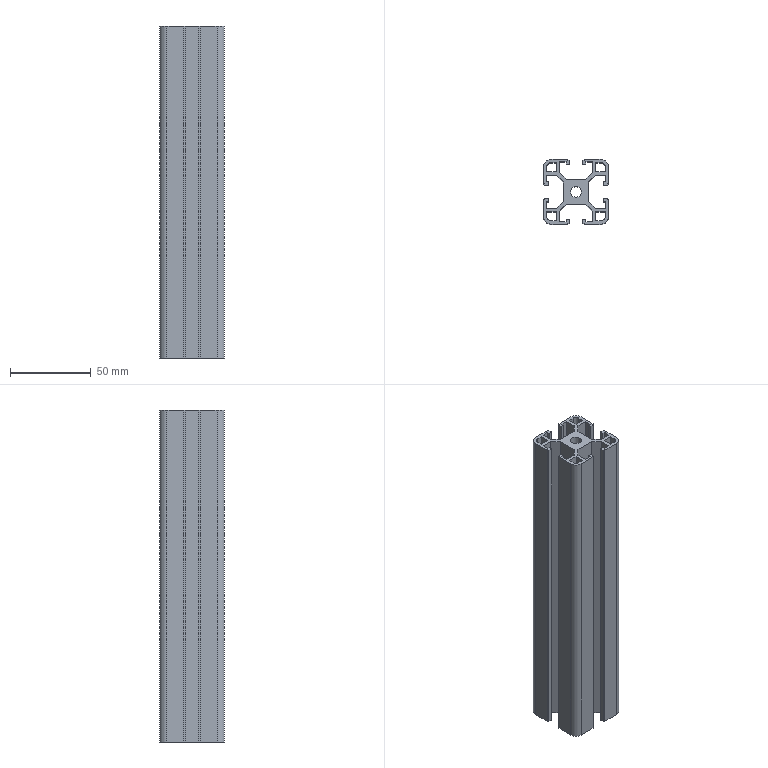Part | NX | features DATUM_CSYS 2, EXTRUDE 1, SKETCH 1 | 1 solid | 103 faces | box 40 x 40 x 205 mm | volume 118192 mm3 | plane 94 | cylinder 9 | commonest cylinder face diameters 5 x4 9 x4 6.8 x1